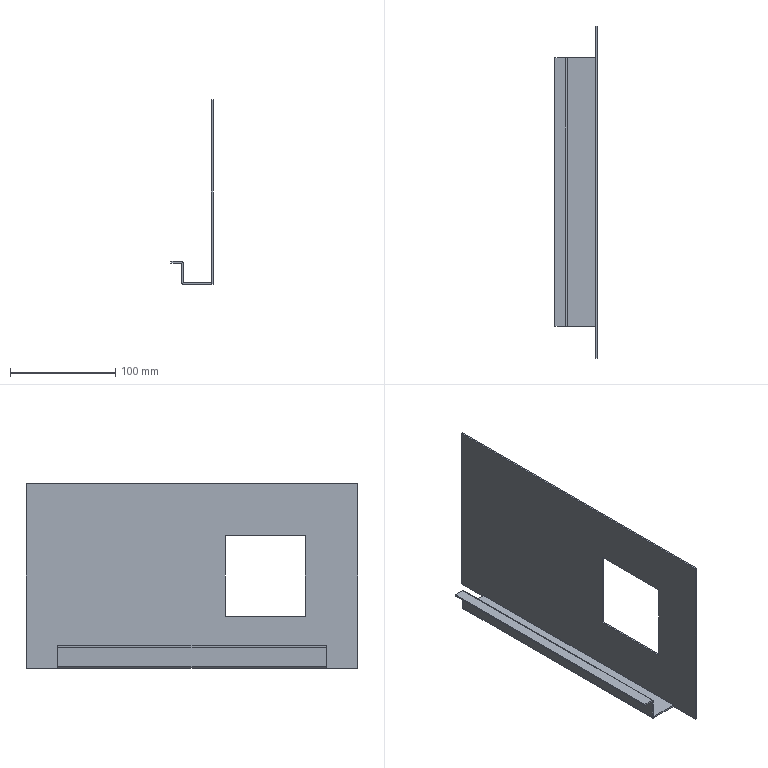Part | 1 solid | 42 faces | box 40 x 315 x 175 mm | volume 95980 mm3 | plane 36 | cylinder 6 | commonest cylinder face diameters 0.2 x3 3.2 x3
STEP:
#1=CARTESIAN_POINT('',(217.5,-127.5,-155.));
#2=VERTEX_POINT('',#1);
#3=CARTESIAN_POINT('',(217.5,-127.5,-153.5));
#4=VERTEX_POINT('',#3);
#5=CARTESIAN_POINT('',(217.5,-127.5,-663.884));
#6=DIRECTION('',(0.,0.,1.));
#7=VECTOR('',#6,1000.);
#8=LINE('',#5,#7);
#9=EDGE_CURVE('',#2,#4,#8,.T.);
#10=ORIENTED_EDGE('',*,*,#9,.T.);
#11=CARTESIAN_POINT('',(217.5,127.5,-153.5));
#12=VERTEX_POINT('',#11);
#13=CARTESIAN_POINT('',(217.5,-127.5,-153.5));
#14=DIRECTION('',(0.,1.,0.));
#15=VECTOR('',#14,1000.);
#16=LINE('',#13,#15);
#17=EDGE_CURVE('',#4,#12,#16,.T.);
#18=ORIENTED_EDGE('',*,*,#17,.T.);
#19=CARTESIAN_POINT('',(217.5,127.5,-155.));
#20=VERTEX_POINT('',#19);
#21=CARTESIAN_POINT('',(217.5,127.5,-663.884));
#22=DIRECTION('',(0.,0.,1.));
#23=VECTOR('',#22,1000.);
#24=LINE('',#21,#23);
#25=EDGE_CURVE('',#20,#12,#24,.T.);
#26=ORIENTED_EDGE('',*,*,#25,.F.);
#27=CARTESIAN_POINT('',(217.5,-127.5,-155.));
#28=DIRECTION('',(0.,1.,0.));
#29=VECTOR('',#28,1000.);
#30=LINE('',#27,#29);
#31=EDGE_CURVE('',#2,#20,#30,.T.);
#32=ORIENTED_EDGE('',*,*,#31,.F.);
#33=EDGE_LOOP('',(#10,#18,#26,#32));
#34=FACE_OUTER_BOUND('',#33,.T.);
#35=CARTESIAN_POINT('',(217.5,-127.5,-663.884));
#36=DIRECTION('',(1.,0.,0.));
#37=DIRECTION('',(0.,-1.,0.));
#38=AXIS2_PLACEMENT_3D('',#35,#36,#37);
#39=PLANE('',#38);
#40=ADVANCED_FACE('',(#34),#39,.F.);
#41=CARTESIAN_POINT('',(227.4,-127.5,-153.5));
#42=VERTEX_POINT('',#41);
#43=CARTESIAN_POINT('',(-2832.5,-127.5,-153.5));
#44=DIRECTION('',(1.,0.,0.));
#45=VECTOR('',#44,1000.);
#46=LINE('',#43,#45);
#47=EDGE_CURVE('',#4,#42,#46,.T.);
#48=ORIENTED_EDGE('',*,*,#47,.F.);
#49=ORIENTED_EDGE('',*,*,#9,.F.);
#50=CARTESIAN_POINT('',(227.4,-127.5,-155.));
#51=VERTEX_POINT('',#50);
#52=CARTESIAN_POINT('',(-2832.5,-127.5,-155.));
#53=DIRECTION('',(1.,0.,0.));
#54=VECTOR('',#53,1000.);
#55=LINE('',#52,#54);
#56=EDGE_CURVE('',#2,#51,#55,.T.);
#57=ORIENTED_EDGE('',*,*,#56,.T.);
#58=CARTESIAN_POINT('',(227.4,-127.5,-663.884));
#59=DIRECTION('',(0.,0.,1.));
#60=VECTOR('',#59,1000.);
#61=LINE('',#58,#60);
#62=EDGE_CURVE('',#51,#42,#61,.T.);
#63=ORIENTED_EDGE('',*,*,#62,.T.);
#64=EDGE_LOOP('',(#48,#49,#57,#63));
#65=FACE_OUTER_BOUND('',#64,.T.);
#66=CARTESIAN_POINT('',(-2832.5,-127.5,-663.884));
#67=DIRECTION('',(0.,-1.,0.));
#68=DIRECTION('',(-1.,0.,0.));
#69=AXIS2_PLACEMENT_3D('',#66,#67,#68);
#70=PLANE('',#69);
#71=ADVANCED_FACE('',(#65),#70,.T.);
#72=ORIENTED_EDGE('',*,*,#47,.T.);
#73=CARTESIAN_POINT('',(227.4,127.5,-153.5));
#74=VERTEX_POINT('',#73);
#75=CARTESIAN_POINT('',(227.4,-127.5,-153.5));
#76=DIRECTION('',(0.,1.,0.));
#77=VECTOR('',#76,1000.);
#78=LINE('',#75,#77);
#79=EDGE_CURVE('',#42,#74,#78,.T.);
#80=ORIENTED_EDGE('',*,*,#79,.T.);
#81=CARTESIAN_POINT('',(2832.5,127.5,-153.5));
#82=DIRECTION('',(-1.,0.,0.));
#83=VECTOR('',#82,1000.);
#84=LINE('',#81,#83);
#85=EDGE_CURVE('',#74,#12,#84,.T.);
#86=ORIENTED_EDGE('',*,*,#85,.T.);
#87=ORIENTED_EDGE('',*,*,#17,.F.);
#88=EDGE_LOOP('',(#72,#80,#86,#87));
#89=FACE_OUTER_BOUND('',#88,.T.);
#90=CARTESIAN_POINT('',(-2832.5,-127.5,-153.5));
#91=DIRECTION('',(0.,0.,-1.));
#92=DIRECTION('',(0.,-1.,0.));
#93=AXIS2_PLACEMENT_3D('',#90,#91,#92);
#94=PLANE('',#93);
#95=ADVANCED_FACE('',(#89),#94,.F.);
#96=ORIENTED_EDGE('',*,*,#85,.F.);
#97=CARTESIAN_POINT('',(227.4,127.5,-155.));
#98=VERTEX_POINT('',#97);
#99=CARTESIAN_POINT('',(227.4,127.5,-663.884));
#100=DIRECTION('',(0.,0.,1.));
#101=VECTOR('',#100,1000.);
#102=LINE('',#99,#101);
#103=EDGE_CURVE('',#98,#74,#102,.T.);
#104=ORIENTED_EDGE('',*,*,#103,.F.);
#105=CARTESIAN_POINT('',(2832.5,127.5,-155.));
#106=DIRECTION('',(-1.,0.,0.));
#107=VECTOR('',#106,1000.);
#108=LINE('',#105,#107);
#109=EDGE_CURVE('',#98,#20,#108,.T.);
#110=ORIENTED_EDGE('',*,*,#109,.T.);
#111=ORIENTED_EDGE('',*,*,#25,.T.);
#112=EDGE_LOOP('',(#96,#104,#110,#111));
#113=FACE_OUTER_BOUND('',#112,.T.);
#114=CARTESIAN_POINT('',(2832.5,127.5,-663.884));
#115=DIRECTION('',(0.,1.,0.));
#116=DIRECTION('',(1.,0.,0.));
#117=AXIS2_PLACEMENT_3D('',#114,#115,#116);
#118=PLANE('',#117);
#119=ADVANCED_FACE('',(#113),#118,.T.);
#120=CARTESIAN_POINT('',(227.4,-127.5,-155.));
#121=DIRECTION('',(0.,1.,0.));
#122=VECTOR('',#121,1000.);
#123=LINE('',#120,#122);
#124=EDGE_CURVE('',#51,#98,#123,.T.);
#125=ORIENTED_EDGE('',*,*,#124,.F.);
#126=ORIENTED_EDGE('',*,*,#56,.F.);
#127=ORIENTED_EDGE('',*,*,#31,.T.);
#128=ORIENTED_EDGE('',*,*,#109,.F.);
#129=EDGE_LOOP('',(#125,#126,#127,#128));
#130=FACE_OUTER_BOUND('',#129,.T.);
#131=CARTESIAN_POINT('',(-2832.5,-127.5,-155.));
#132=DIRECTION('',(0.,0.,-1.));
#133=DIRECTION('',(0.,-1.,0.));
#134=AXIS2_PLACEMENT_3D('',#131,#132,#133);
#135=PLANE('',#134);
#136=ADVANCED_FACE('',(#130),#135,.T.);
#137=CARTESIAN_POINT('',(227.5,-127.5,-173.4));
#138=VERTEX_POINT('',#137);
#139=CARTESIAN_POINT('',(227.5,-127.5,-155.1));
#140=VERTEX_POINT('',#139);
#141=CARTESIAN_POINT('',(227.5,-127.5,-175.));
#142=DIRECTION('',(0.,0.,1.));
#143=VECTOR('',#142,1000.);
#144=LINE('',#141,#143);
#145=EDGE_CURVE('',#138,#140,#144,.T.);
#146=ORIENTED_EDGE('',*,*,#145,.F.);
#147=CARTESIAN_POINT('',(229.,-127.5,-173.4));
#148=VERTEX_POINT('',#147);
#149=CARTESIAN_POINT('',(740.312,-127.5,-173.4));
#150=DIRECTION('',(-1.,0.,0.));
#151=VECTOR('',#150,1000.);
#152=LINE('',#149,#151);
#153=EDGE_CURVE('',#148,#138,#152,.T.);
#154=ORIENTED_EDGE('',*,*,#153,.F.);
#155=CARTESIAN_POINT('',(229.,-127.5,-155.1));
#156=VERTEX_POINT('',#155);
#157=CARTESIAN_POINT('',(229.,-127.5,-175.));
#158=DIRECTION('',(0.,0.,-1.));
#159=VECTOR('',#158,1000.);
#160=LINE('',#157,#159);
#161=EDGE_CURVE('',#156,#148,#160,.T.);
#162=ORIENTED_EDGE('',*,*,#161,.F.);
#163=CARTESIAN_POINT('',(740.312,-127.5,-155.1));
#164=DIRECTION('',(-1.,0.,0.));
#165=VECTOR('',#164,1000.);
#166=LINE('',#163,#165);
#167=EDGE_CURVE('',#156,#140,#166,.T.);
#168=ORIENTED_EDGE('',*,*,#167,.T.);
#169=EDGE_LOOP('',(#146,#154,#162,#168));
#170=FACE_OUTER_BOUND('',#169,.T.);
#171=CARTESIAN_POINT('',(740.312,-127.5,-175.));
#172=DIRECTION('',(0.,1.,0.));
#173=DIRECTION('',(0.,0.,-1.));
#174=AXIS2_PLACEMENT_3D('',#171,#172,#173);
#175=PLANE('',#174);
#176=ADVANCED_FACE('',(#170),#175,.F.);
#177=CARTESIAN_POINT('',(227.5,127.5,-155.1));
#178=VERTEX_POINT('',#177);
#179=CARTESIAN_POINT('',(227.5,127.5,-173.4));
#180=VERTEX_POINT('',#179);
#181=CARTESIAN_POINT('',(227.5,127.5,-175.));
#182=DIRECTION('',(0.,0.,-1.));
#183=VECTOR('',#182,1000.);
#184=LINE('',#181,#183);
#185=EDGE_CURVE('',#178,#180,#184,.T.);
#186=ORIENTED_EDGE('',*,*,#185,.F.);
#187=CARTESIAN_POINT('',(229.,127.5,-155.1));
#188=VERTEX_POINT('',#187);
#189=CARTESIAN_POINT('',(740.312,127.5,-155.1));
#190=DIRECTION('',(-1.,0.,0.));
#191=VECTOR('',#190,1000.);
#192=LINE('',#189,#191);
#193=EDGE_CURVE('',#188,#178,#192,.T.);
#194=ORIENTED_EDGE('',*,*,#193,.F.);
#195=CARTESIAN_POINT('',(229.,127.5,-173.4));
#196=VERTEX_POINT('',#195);
#197=CARTESIAN_POINT('',(229.,127.5,-175.));
#198=DIRECTION('',(0.,0.,-1.));
#199=VECTOR('',#198,1000.);
#200=LINE('',#197,#199);
#201=EDGE_CURVE('',#188,#196,#200,.T.);
#202=ORIENTED_EDGE('',*,*,#201,.T.);
#203=CARTESIAN_POINT('',(740.312,127.5,-173.4));
#204=DIRECTION('',(-1.,0.,0.));
#205=VECTOR('',#204,1000.);
#206=LINE('',#203,#205);
#207=EDGE_CURVE('',#196,#180,#206,.T.);
#208=ORIENTED_EDGE('',*,*,#207,.T.);
#209=EDGE_LOOP('',(#186,#194,#202,#208));
#210=FACE_OUTER_BOUND('',#209,.T.);
#211=CARTESIAN_POINT('',(740.312,127.5,-175.));
#212=DIRECTION('',(0.,-1.,0.));
#213=DIRECTION('',(0.,0.,1.));
#214=AXIS2_PLACEMENT_3D('',#211,#212,#213);
#215=PLANE('',#214);
#216=ADVANCED_FACE('',(#210),#215,.F.);
#217=ORIENTED_EDGE('',*,*,#201,.F.);
#218=CARTESIAN_POINT('',(229.,-127.5,-155.1));
#219=DIRECTION('',(0.,-1.,0.));
#220=VECTOR('',#219,1000.);
#221=LINE('',#218,#220);
#222=EDGE_CURVE('',#188,#156,#221,.T.);
#223=ORIENTED_EDGE('',*,*,#222,.T.);
#224=ORIENTED_EDGE('',*,*,#161,.T.);
#225=CARTESIAN_POINT('',(229.,127.5,-173.4));
#226=DIRECTION('',(0.,1.,0.));
#227=VECTOR('',#226,1000.);
#228=LINE('',#225,#227);
#229=EDGE_CURVE('',#148,#196,#228,.T.);
#230=ORIENTED_EDGE('',*,*,#229,.T.);
#231=EDGE_LOOP('',(#217,#223,#224,#230));
#232=FACE_OUTER_BOUND('',#231,.T.);
#233=CARTESIAN_POINT('',(229.,-2732.5,-175.));
#234=DIRECTION('',(-1.,0.,0.));
#235=DIRECTION('',(0.,0.,-1.));
#236=AXIS2_PLACEMENT_3D('',#233,#234,#235);
#237=PLANE('',#236);
#238=ADVANCED_FACE('',(#232),#237,.F.);
#239=CARTESIAN_POINT('',(227.5,-127.5,-155.1));
#240=DIRECTION('',(0.,-1.,0.));
#241=VECTOR('',#240,1000.);
#242=LINE('',#239,#241);
#243=EDGE_CURVE('',#178,#140,#242,.T.);
#244=ORIENTED_EDGE('',*,*,#243,.F.);
#245=ORIENTED_EDGE('',*,*,#185,.T.);
#246=CARTESIAN_POINT('',(227.5,127.5,-173.4));
#247=DIRECTION('',(0.,1.,0.));
#248=VECTOR('',#247,1000.);
#249=LINE('',#246,#248);
#250=EDGE_CURVE('',#138,#180,#249,.T.);
#251=ORIENTED_EDGE('',*,*,#250,.F.);
#252=ORIENTED_EDGE('',*,*,#145,.T.);
#253=EDGE_LOOP('',(#244,#245,#251,#252));
#254=FACE_OUTER_BOUND('',#253,.T.);
#255=CARTESIAN_POINT('',(227.5,-127.5,-175.));
#256=DIRECTION('',(-1.,0.,0.));
#257=DIRECTION('',(0.,0.,1.));
#258=AXIS2_PLACEMENT_3D('',#255,#256,#257);
#259=PLANE('',#258);
#260=ADVANCED_FACE('',(#254),#259,.T.);
#261=CARTESIAN_POINT('',(256.,127.65,-173.25));
#262=VERTEX_POINT('',#261);
#263=CARTESIAN_POINT('',(257.5,127.65,-173.25));
#264=VERTEX_POINT('',#263);
#265=CARTESIAN_POINT('',(-464.694,127.65,-173.25));
#266=DIRECTION('',(1.,0.,0.));
#267=VECTOR('',#266,1000.);
#268=LINE('',#265,#267);
#269=EDGE_CURVE('',#262,#264,#268,.T.);
#270=ORIENTED_EDGE('',*,*,#269,.T.);
#271=CARTESIAN_POINT('',(257.5,127.5,-173.25));
#272=VERTEX_POINT('',#271);
#273=CARTESIAN_POINT('',(257.5,-2732.5,-173.25));
#274=DIRECTION('',(0.,-1.,0.));
#275=VECTOR('',#274,1000.);
#276=LINE('',#273,#275);
#277=EDGE_CURVE('',#264,#272,#276,.T.);
#278=ORIENTED_EDGE('',*,*,#277,.T.);
#279=CARTESIAN_POINT('',(256.,127.5,-173.25));
#280=VERTEX_POINT('',#279);
#281=CARTESIAN_POINT('',(-464.694,127.5,-173.25));
#282=DIRECTION('',(1.,0.,0.));
#283=VECTOR('',#282,1000.);
#284=LINE('',#281,#283);
#285=EDGE_CURVE('',#280,#272,#284,.T.);
#286=ORIENTED_EDGE('',*,*,#285,.F.);
#287=CARTESIAN_POINT('',(256.,-156.3,-173.25));
#288=DIRECTION('',(0.,-1.,0.));
#289=VECTOR('',#288,1000.);
#290=LINE('',#287,#289);
#291=EDGE_CURVE('',#262,#280,#290,.T.);
#292=ORIENTED_EDGE('',*,*,#291,.F.);
#293=EDGE_LOOP('',(#270,#278,#286,#292));
#294=FACE_OUTER_BOUND('',#293,.T.);
#295=CARTESIAN_POINT('',(-464.694,-156.3,-173.25));
#296=DIRECTION('',(0.,0.,1.));
#297=DIRECTION('',(0.,-1.,0.));
#298=AXIS2_PLACEMENT_3D('',#295,#296,#297);
#299=PLANE('',#298);
#300=ADVANCED_FACE('',(#294),#299,.F.);
#301=CARTESIAN_POINT('',(256.,127.65,-175.));
#302=VERTEX_POINT('',#301);
#303=CARTESIAN_POINT('',(257.5,127.65,-175.));
#304=VERTEX_POINT('',#303);
#305=CARTESIAN_POINT('',(-464.694,127.65,-175.));
#306=DIRECTION('',(1.,0.,0.));
#307=VECTOR('',#306,1000.);
#308=LINE('',#305,#307);
#309=EDGE_CURVE('',#302,#304,#308,.T.);
#310=ORIENTED_EDGE('',*,*,#309,.T.);
#311=CARTESIAN_POINT('',(257.5,127.65,-173.063));
#312=DIRECTION('',(0.,0.,1.));
#313=VECTOR('',#312,1000.);
#314=LINE('',#311,#313);
#315=EDGE_CURVE('',#304,#264,#314,.T.);
#316=ORIENTED_EDGE('',*,*,#315,.T.);
#317=ORIENTED_EDGE('',*,*,#269,.F.);
#318=CARTESIAN_POINT('',(256.,127.65,-173.8));
#319=DIRECTION('',(0.,0.,1.));
#320=VECTOR('',#319,1000.);
#321=LINE('',#318,#320);
#322=EDGE_CURVE('',#302,#262,#321,.T.);
#323=ORIENTED_EDGE('',*,*,#322,.F.);
#324=EDGE_LOOP('',(#310,#316,#317,#323));
#325=FACE_OUTER_BOUND('',#324,.T.);
#326=CARTESIAN_POINT('',(-464.694,127.65,-173.8));
#327=DIRECTION('',(0.,1.,0.));
#328=DIRECTION('',(0.,0.,1.));
#329=AXIS2_PLACEMENT_3D('',#326,#327,#328);
#330=PLANE('',#329);
#331=ADVANCED_FACE('',(#325),#330,.F.);
#332=CARTESIAN_POINT('',(257.5,157.5,-175.));
#333=VERTEX_POINT('',#332);
#334=CARTESIAN_POINT('',(257.5,-2732.5,-175.));
#335=DIRECTION('',(0.,1.,0.));
#336=VECTOR('',#335,1000.);
#337=LINE('',#334,#336);
#338=EDGE_CURVE('',#304,#333,#337,.T.);
#339=ORIENTED_EDGE('',*,*,#338,.F.);
#340=ORIENTED_EDGE('',*,*,#309,.F.);
#341=CARTESIAN_POINT('',(256.,157.5,-175.));
#342=VERTEX_POINT('',#341);
#343=CARTESIAN_POINT('',(256.,2732.5,-175.));
#344=DIRECTION('',(0.,1.,0.));
#345=VECTOR('',#344,1000.);
#346=LINE('',#343,#345);
#347=EDGE_CURVE('',#302,#342,#346,.T.);
#348=ORIENTED_EDGE('',*,*,#347,.T.);
#349=CARTESIAN_POINT('',(-464.694,157.5,-175.));
#350=DIRECTION('',(1.,0.,0.));
#351=VECTOR('',#350,1000.);
#352=LINE('',#349,#351);
#353=EDGE_CURVE('',#342,#333,#352,.T.);
#354=ORIENTED_EDGE('',*,*,#353,.T.);
#355=EDGE_LOOP('',(#339,#340,#348,#354));
#356=FACE_OUTER_BOUND('',#355,.T.);
#357=CARTESIAN_POINT('',(-464.694,2732.5,-175.));
#358=DIRECTION('',(0.,0.,-1.));
#359=DIRECTION('',(-1.,0.,0.));
#360=AXIS2_PLACEMENT_3D('',#357,#358,#359);
#361=PLANE('',#360);
#362=ADVANCED_FACE('',(#356),#361,.T.);
#363=CARTESIAN_POINT('',(256.,157.5,0.));
#364=VERTEX_POINT('',#363);
#365=CARTESIAN_POINT('',(257.5,157.5,0.));
#366=VERTEX_POINT('',#365);
#367=CARTESIAN_POINT('',(-464.694,157.5,0.));
#368=DIRECTION('',(1.,0.,0.));
#369=VECTOR('',#368,1000.);
#370=LINE('',#367,#369);
#371=EDGE_CURVE('',#364,#366,#370,.T.);
#372=ORIENTED_EDGE('',*,*,#371,.T.);
#373=CARTESIAN_POINT('',(257.5,157.5,-173.063));
#374=DIRECTION('',(0.,0.,-1.));
#375=VECTOR('',#374,1000.);
#376=LINE('',#373,#375);
#377=EDGE_CURVE('',#366,#333,#376,.T.);
#378=ORIENTED_EDGE('',*,*,#377,.T.);
#379=ORIENTED_EDGE('',*,*,#353,.F.);
#380=CARTESIAN_POINT('',(256.,157.5,-173.063));
#381=DIRECTION('',(0.,0.,-1.));
#382=VECTOR('',#381,1000.);
#383=LINE('',#380,#382);
#384=EDGE_CURVE('',#364,#342,#383,.T.);
#385=ORIENTED_EDGE('',*,*,#384,.F.);
#386=EDGE_LOOP('',(#372,#378,#379,#385));
#387=FACE_OUTER_BOUND('',#386,.T.);
#388=CARTESIAN_POINT('',(-464.694,157.5,-173.063));
#389=DIRECTION('',(0.,-1.,0.));
#390=DIRECTION('',(1.,0.,0.));
#391=AXIS2_PLACEMENT_3D('',#388,#389,#390);
#392=PLANE('',#391);
#393=ADVANCED_FACE('',(#387),#392,.F.);
#394=CARTESIAN_POINT('',(257.5,-157.5,0.));
#395=VERTEX_POINT('',#394);
#396=CARTESIAN_POINT('',(257.5,-2732.5,0.));
#397=DIRECTION('',(0.,1.,0.));
#398=VECTOR('',#397,1000.);
#399=LINE('',#396,#398);
#400=EDGE_CURVE('',#395,#366,#399,.T.);
#401=ORIENTED_EDGE('',*,*,#400,.T.);
#402=ORIENTED_EDGE('',*,*,#371,.F.);
#403=CARTESIAN_POINT('',(256.,-157.5,0.));
#404=VERTEX_POINT('',#403);
#405=CARTESIAN_POINT('',(256.,0.,0.));
#406=DIRECTION('',(0.,-1.,0.));
#407=VECTOR('',#406,1000.);
#408=LINE('',#405,#407);
#409=EDGE_CURVE('',#364,#404,#408,.T.);
#410=ORIENTED_EDGE('',*,*,#409,.T.);
#411=CARTESIAN_POINT('',(-464.694,-157.5,0.));
#412=DIRECTION('',(1.,0.,0.));
#413=VECTOR('',#412,1000.);
#414=LINE('',#411,#413);
#415=EDGE_CURVE('',#404,#395,#414,.T.);
#416=ORIENTED_EDGE('',*,*,#415,.T.);
#417=EDGE_LOOP('',(#401,#402,#410,#416));
#418=FACE_OUTER_BOUND('',#417,.T.);
#419=CARTESIAN_POINT('',(-464.694,0.,0.));
#420=DIRECTION('',(0.,0.,1.));
#421=DIRECTION('',(1.,0.,0.));
#422=AXIS2_PLACEMENT_3D('',#419,#420,#421);
#423=PLANE('',#422);
#424=ADVANCED_FACE('',(#418),#423,.T.);
#425=CARTESIAN_POINT('',(256.,-157.5,-175.));
#426=VERTEX_POINT('',#425);
#427=CARTESIAN_POINT('',(257.5,-157.5,-175.));
#428=VERTEX_POINT('',#427);
#429=CARTESIAN_POINT('',(-464.694,-157.5,-175.));
#430=DIRECTION('',(1.,0.,0.));
#431=VECTOR('',#430,1000.);
#432=LINE('',#429,#431);
#433=EDGE_CURVE('',#426,#428,#432,.T.);
#434=ORIENTED_EDGE('',*,*,#433,.T.);
#435=CARTESIAN_POINT('',(257.5,-157.5,-173.063));
#436=DIRECTION('',(0.,0.,-1.));
#437=VECTOR('',#436,1000.);
#438=LINE('',#435,#437);
#439=EDGE_CURVE('',#395,#428,#438,.T.);
#440=ORIENTED_EDGE('',*,*,#439,.F.);
#441=ORIENTED_EDGE('',*,*,#415,.F.);
#442=CARTESIAN_POINT('',(256.,-157.5,-173.063));
#443=DIRECTION('',(0.,0.,1.));
#444=VECTOR('',#443,1000.);
#445=LINE('',#442,#444);
#446=EDGE_CURVE('',#426,#404,#445,.T.);
#447=ORIENTED_EDGE('',*,*,#446,.F.);
#448=EDGE_LOOP('',(#434,#440,#441,#447));
#449=FACE_OUTER_BOUND('',#448,.T.);
#450=CARTESIAN_POINT('',(-464.694,-157.5,-173.063));
#451=DIRECTION('',(0.,1.,0.));
#452=DIRECTION('',(-1.,0.,0.));
#453=AXIS2_PLACEMENT_3D('',#450,#451,#452);
#454=PLANE('',#453);
#455=ADVANCED_FACE('',(#449),#454,.F.);
#456=CARTESIAN_POINT('',(257.5,-127.65,-175.));
#457=VERTEX_POINT('',#456);
#458=CARTESIAN_POINT('',(257.5,-2732.5,-175.));
#459=DIRECTION('',(0.,1.,0.));
#460=VECTOR('',#459,1000.);
#461=LINE('',#458,#460);
#462=EDGE_CURVE('',#428,#457,#461,.T.);
#463=ORIENTED_EDGE('',*,*,#462,.F.);
#464=ORIENTED_EDGE('',*,*,#433,.F.);
#465=CARTESIAN_POINT('',(256.,-127.65,-175.));
#466=VERTEX_POINT('',#465);
#467=CARTESIAN_POINT('',(256.,2732.5,-175.));
#468=DIRECTION('',(0.,1.,0.));
#469=VECTOR('',#468,1000.);
#470=LINE('',#467,#469);
#471=EDGE_CURVE('',#426,#466,#470,.T.);
#472=ORIENTED_EDGE('',*,*,#471,.T.);
#473=CARTESIAN_POINT('',(-464.694,-127.65,-175.));
#474=DIRECTION('',(1.,0.,0.));
#475=VECTOR('',#474,1000.);
#476=LINE('',#473,#475);
#477=EDGE_CURVE('',#466,#457,#476,.T.);
#478=ORIENTED_EDGE('',*,*,#477,.T.);
#479=EDGE_LOOP('',(#463,#464,#472,#478));
#480=FACE_OUTER_BOUND('',#479,.T.);
#481=CARTESIAN_POINT('',(-464.694,2732.5,-175.));
#482=DIRECTION('',(0.,0.,-1.));
#483=DIRECTION('',(-1.,0.,0.));
#484=AXIS2_PLACEMENT_3D('',#481,#482,#483);
#485=PLANE('',#484);
#486=ADVANCED_FACE('',(#480),#485,.T.);
#487=CARTESIAN_POINT('',(256.,-127.65,-173.25));
#488=VERTEX_POINT('',#487);
#489=CARTESIAN_POINT('',(257.5,-127.65,-173.25));
#490=VERTEX_POINT('',#489);
#491=CARTESIAN_POINT('',(-464.694,-127.65,-173.25));
#492=DIRECTION('',(1.,0.,0.));
#493=VECTOR('',#492,1000.);
#494=LINE('',#491,#493);
#495=EDGE_CURVE('',#488,#490,#494,.T.);
#496=ORIENTED_EDGE('',*,*,#495,.T.);
#497=CARTESIAN_POINT('',(257.5,-127.65,-173.063));
#498=DIRECTION('',(0.,0.,-1.));
#499=VECTOR('',#498,1000.);
#500=LINE('',#497,#499);
#501=EDGE_CURVE('',#490,#457,#500,.T.);
#502=ORIENTED_EDGE('',*,*,#501,.T.);
#503=ORIENTED_EDGE('',*,*,#477,.F.);
#504=CARTESIAN_POINT('',(256.,-127.65,-173.8));
#505=DIRECTION('',(0.,0.,-1.));
#506=VECTOR('',#505,1000.);
#507=LINE('',#504,#506);
#508=EDGE_CURVE('',#488,#466,#507,.T.);
#509=ORIENTED_EDGE('',*,*,#508,.F.);
#510=EDGE_LOOP('',(#496,#502,#503,#509));
#511=FACE_OUTER_BOUND('',#510,.T.);
#512=CARTESIAN_POINT('',(-464.694,-127.65,-173.8));
#513=DIRECTION('',(0.,-1.,0.));
#514=DIRECTION('',(0.,0.,-1.));
#515=AXIS2_PLACEMENT_3D('',#512,#513,#514);
#516=PLANE('',#515);
#517=ADVANCED_FACE('',(#511),#516,.F.);
#518=CARTESIAN_POINT('',(256.,-127.5,-173.25));
#519=VERTEX_POINT('',#518);
#520=CARTESIAN_POINT('',(257.5,-127.5,-173.25));
#521=VERTEX_POINT('',#520);
#522=CARTESIAN_POINT('',(-464.694,-127.5,-173.25));
#523=DIRECTION('',(1.,0.,0.));
#524=VECTOR('',#523,1000.);
#525=LINE('',#522,#524);
#526=EDGE_CURVE('',#519,#521,#525,.T.);
#527=ORIENTED_EDGE('',*,*,#526,.T.);
#528=CARTESIAN_POINT('',(257.5,-2732.5,-173.25));
#529=DIRECTION('',(0.,-1.,0.));
#530=VECTOR('',#529,1000.);
#531=LINE('',#528,#530);
#532=EDGE_CURVE('',#521,#490,#531,.T.);
#533=ORIENTED_EDGE('',*,*,#532,.T.);
#534=ORIENTED_EDGE('',*,*,#495,.F.);
#535=CARTESIAN_POINT('',(256.,-156.3,-173.25));
#536=DIRECTION('',(0.,-1.,0.));
#537=VECTOR('',#536,1000.);
#538=LINE('',#535,#537);
#539=EDGE_CURVE('',#519,#488,#538,.T.);
#540=ORIENTED_EDGE('',*,*,#539,.F.);
#541=EDGE_LOOP('',(#527,#533,#534,#540));
#542=FACE_OUTER_BOUND('',#541,.T.);
#543=CARTESIAN_POINT('',(-464.694,-156.3,-173.25));
#544=DIRECTION('',(0.,0.,1.));
#545=DIRECTION('',(0.,-1.,0.));
#546=AXIS2_PLACEMENT_3D('',#543,#544,#545);
#547=PLANE('',#546);
#548=ADVANCED_FACE('',(#542),#547,.F.);
#549=CARTESIAN_POINT('',(257.5,-107.5,-49.5));
#550=VERTEX_POINT('',#549);
#551=CARTESIAN_POINT('',(257.5,-107.5,-125.5));
#552=VERTEX_POINT('',#551);
#553=CARTESIAN_POINT('',(257.5,-107.5,-125.5));
#554=DIRECTION('',(0.,0.,-1.));
#555=VECTOR('',#554,1000.);
#556=LINE('',#553,#555);
#557=EDGE_CURVE('',#550,#552,#556,.T.);
#558=ORIENTED_EDGE('',*,*,#557,.T.);
#559=CARTESIAN_POINT('',(256.,-107.5,-125.5));
#560=VERTEX_POINT('',#559);
#561=CARTESIAN_POINT('',(256.3,-107.5,-125.5));
#562=DIRECTION('',(1.,0.,0.));
#563=VECTOR('',#562,1000.);
#564=LINE('',#561,#563);
#565=EDGE_CURVE('',#560,#552,#564,.T.);
#566=ORIENTED_EDGE('',*,*,#565,.F.);
#567=CARTESIAN_POINT('',(256.,-107.5,-49.5));
#568=VERTEX_POINT('',#567);
#569=CARTESIAN_POINT('',(256.,-107.5,-125.5));
#570=DIRECTION('',(0.,0.,-1.));
#571=VECTOR('',#570,1000.);
#572=LINE('',#569,#571);
#573=EDGE_CURVE('',#568,#560,#572,.T.);
#574=ORIENTED_EDGE('',*,*,#573,.F.);
#575=CARTESIAN_POINT('',(256.3,-107.5,-49.5));
#576=DIRECTION('',(1.,0.,0.));
#577=VECTOR('',#576,1000.);
#578=LINE('',#575,#577);
#579=EDGE_CURVE('',#568,#550,#578,.T.);
#580=ORIENTED_EDGE('',*,*,#579,.T.);
#581=EDGE_LOOP('',(#558,#566,#574,#580));
#582=FACE_OUTER_BOUND('',#581,.T.);
#583=CARTESIAN_POINT('',(256.3,-107.5,-125.5));
#584=DIRECTION('',(0.,-1.,0.));
#585=DIRECTION('',(0.,0.,-1.));
#586=AXIS2_PLACEMENT_3D('',#583,#584,#585);
#587=PLANE('',#586);
#588=ADVANCED_FACE('',(#582),#587,.F.);
#589=CARTESIAN_POINT('',(257.5,-31.5,-49.5));
#590=VERTEX_POINT('',#589);
#591=CARTESIAN_POINT('',(257.5,-107.5,-49.5));
#592=DIRECTION('',(0.,-1.,0.));
#593=VECTOR('',#592,1000.);
#594=LINE('',#591,#593);
#595=EDGE_CURVE('',#590,#550,#594,.T.);
#596=ORIENTED_EDGE('',*,*,#595,.T.);
#597=ORIENTED_EDGE('',*,*,#579,.F.);
#598=CARTESIAN_POINT('',(256.,-31.5,-49.5));
#599=VERTEX_POINT('',#598);
#600=CARTESIAN_POINT('',(256.,-107.5,-49.5));
#601=DIRECTION('',(0.,-1.,0.));
#602=VECTOR('',#601,1000.);
#603=LINE('',#600,#602);
#604=EDGE_CURVE('',#599,#568,#603,.T.);
#605=ORIENTED_EDGE('',*,*,#604,.F.);
#606=CARTESIAN_POINT('',(256.3,-31.5,-49.5));
#607=DIRECTION('',(1.,0.,0.));
#608=VECTOR('',#607,1000.);
#609=LINE('',#606,#608);
#610=EDGE_CURVE('',#599,#590,#609,.T.);
#611=ORIENTED_EDGE('',*,*,#610,.T.);
#612=EDGE_LOOP('',(#596,#597,#605,#611));
#613=FACE_OUTER_BOUND('',#612,.T.);
#614=CARTESIAN_POINT('',(256.3,-107.5,-49.5));
#615=DIRECTION('',(0.,0.,1.));
#616=DIRECTION('',(0.,-1.,0.));
#617=AXIS2_PLACEMENT_3D('',#614,#615,#616);
#618=PLANE('',#617);
#619=ADVANCED_FACE('',(#613),#618,.F.);
#620=CARTESIAN_POINT('',(257.5,-31.5,-125.5));
#621=VERTEX_POINT('',#620);
#622=CARTESIAN_POINT('',(257.5,-31.5,-125.5));
#623=DIRECTION('',(0.,0.,1.));
#624=VECTOR('',#623,1000.);
#625=LINE('',#622,#624);
#626=EDGE_CURVE('',#621,#590,#625,.T.);
#627=ORIENTED_EDGE('',*,*,#626,.T.);
#628=ORIENTED_EDGE('',*,*,#610,.F.);
#629=CARTESIAN_POINT('',(256.,-31.5,-125.5));
#630=VERTEX_POINT('',#629);
#631=CARTESIAN_POINT('',(256.,-31.5,-125.5));
#632=DIRECTION('',(0.,0.,1.));
#633=VECTOR('',#632,1000.);
#634=LINE('',#631,#633);
#635=EDGE_CURVE('',#630,#599,#634,.T.);
#636=ORIENTED_EDGE('',*,*,#635,.F.);
#637=CARTESIAN_POINT('',(256.3,-31.5,-125.5));
#638=DIRECTION('',(1.,0.,0.));
#639=VECTOR('',#638,1000.);
#640=LINE('',#637,#639);
#641=EDGE_CURVE('',#630,#621,#640,.T.);
#642=ORIENTED_EDGE('',*,*,#641,.T.);
#643=EDGE_LOOP('',(#627,#628,#636,#642));
#644=FACE_OUTER_BOUND('',#643,.T.);
#645=CARTESIAN_POINT('',(256.3,-31.5,-125.5));
#646=DIRECTION('',(0.,1.,0.));
#647=DIRECTION('',(0.,0.,1.));
#648=AXIS2_PLACEMENT_3D('',#645,#646,#647);
#649=PLANE('',#648);
#650=ADVANCED_FACE('',(#644),#649,.F.);
#651=CARTESIAN_POINT('',(257.5,-107.5,-125.5));
#652=DIRECTION('',(0.,1.,0.));
#653=VECTOR('',#652,1000.);
#654=LINE('',#651,#653);
#655=EDGE_CURVE('',#552,#621,#654,.T.);
#656=ORIENTED_EDGE('',*,*,#655,.T.);
#657=ORIENTED_EDGE('',*,*,#641,.F.);
#658=CARTESIAN_POINT('',(256.,-107.5,-125.5));
#659=DIRECTION('',(0.,1.,0.));
#660=VECTOR('',#659,1000.);
#661=LINE('',#658,#660);
#662=EDGE_CURVE('',#560,#630,#661,.T.);
#663=ORIENTED_EDGE('',*,*,#662,.F.);
#664=ORIENTED_EDGE('',*,*,#565,.T.);
#665=EDGE_LOOP('',(#656,#657,#663,#664));
#666=FACE_OUTER_BOUND('',#665,.T.);
#667=CARTESIAN_POINT('',(256.3,-107.5,-125.5));
#668=DIRECTION('',(0.,0.,-1.));
#669=DIRECTION('',(-1.,0.,0.));
#670=AXIS2_PLACEMENT_3D('',#667,#668,#669);
#671=PLANE('',#670);
#672=ADVANCED_FACE('',(#666),#671,.F.);
#673=ORIENTED_EDGE('',*,*,#285,.T.);
#674=CARTESIAN_POINT('',(257.5,127.5,-173.4));
#675=VERTEX_POINT('',#674);
#676=CARTESIAN_POINT('',(257.5,127.5,-173.063));
#677=DIRECTION('',(0.,0.,-1.));
#678=VECTOR('',#677,1000.);
#679=LINE('',#676,#678);
#680=EDGE_CURVE('',#272,#675,#679,.T.);
#681=ORIENTED_EDGE('',*,*,#680,.T.);
#682=CARTESIAN_POINT('',(256.,127.5,-173.4));
#683=VERTEX_POINT('',#682);
#684=CARTESIAN_POINT('',(-464.694,127.5,-173.4));
#685=DIRECTION('',(1.,0.,0.));
#686=VECTOR('',#685,1000.);
#687=LINE('',#684,#686);
#688=EDGE_CURVE('',#683,#675,#687,.T.);
#689=ORIENTED_EDGE('',*,*,#688,.F.);
#690=CARTESIAN_POINT('',(256.,127.5,-173.8));
#691=DIRECTION('',(0.,0.,-1.));
#692=VECTOR('',#691,1000.);
#693=LINE('',#690,#692);
#694=EDGE_CURVE('',#280,#683,#693,.T.);
#695=ORIENTED_EDGE('',*,*,#694,.F.);
#696=EDGE_LOOP('',(#673,#681,#689,#695));
#697=FACE_OUTER_BOUND('',#696,.T.);
#698=CARTESIAN_POINT('',(-464.694,127.5,-173.8));
#699=DIRECTION('',(0.,-1.,0.));
#700=DIRECTION('',(0.,0.,-1.));
#701=AXIS2_PLACEMENT_3D('',#698,#699,#700);
#702=PLANE('',#701);
#703=ADVANCED_FACE('',(#697),#702,.F.);
#704=ORIENTED_EDGE('',*,*,#626,.F.);
#705=ORIENTED_EDGE('',*,*,#655,.F.);
#706=ORIENTED_EDGE('',*,*,#557,.F.);
#707=ORIENTED_EDGE('',*,*,#595,.F.);
#708=EDGE_LOOP('',(#704,#705,#706,#707));
#709=FACE_BOUND('',#708,.T.);
#710=CARTESIAN_POINT('',(257.5,-127.5,-173.4));
#711=VERTEX_POINT('',#710);
#712=CARTESIAN_POINT('',(257.5,127.5,-173.4));
#713=DIRECTION('',(0.,-1.,0.));
#714=VECTOR('',#713,1000.);
#715=LINE('',#712,#714);
#716=EDGE_CURVE('',#675,#711,#715,.T.);
#717=ORIENTED_EDGE('',*,*,#716,.F.);
#718=ORIENTED_EDGE('',*,*,#680,.F.);
#719=ORIENTED_EDGE('',*,*,#277,.F.);
#720=ORIENTED_EDGE('',*,*,#315,.F.);
#721=ORIENTED_EDGE('',*,*,#338,.T.);
#722=ORIENTED_EDGE('',*,*,#377,.F.);
#723=ORIENTED_EDGE('',*,*,#400,.F.);
#724=ORIENTED_EDGE('',*,*,#439,.T.);
#725=ORIENTED_EDGE('',*,*,#462,.T.);
#726=ORIENTED_EDGE('',*,*,#501,.F.);
#727=ORIENTED_EDGE('',*,*,#532,.F.);
#728=CARTESIAN_POINT('',(257.5,-127.5,-173.063));
#729=DIRECTION('',(0.,0.,1.));
#730=VECTOR('',#729,1000.);
#731=LINE('',#728,#730);
#732=EDGE_CURVE('',#711,#521,#731,.T.);
#733=ORIENTED_EDGE('',*,*,#732,.F.);
#734=EDGE_LOOP('',(#717,#718,#719,#720,#721,#722,#723,#724,#725,#726,#727,#733));
#735=FACE_OUTER_BOUND('',#734,.T.);
#736=CARTESIAN_POINT('',(257.5,-2732.5,-173.063));
#737=DIRECTION('',(-1.,0.,0.));
#738=DIRECTION('',(0.,-1.,0.));
#739=AXIS2_PLACEMENT_3D('',#736,#737,#738);
#740=PLANE('',#739);
#741=ADVANCED_FACE('',(#709,#735),#740,.F.);
#742=CARTESIAN_POINT('',(256.,-127.5,-173.4));
#743=VERTEX_POINT('',#742);
#744=CARTESIAN_POINT('',(-464.694,-127.5,-173.4));
#745=DIRECTION('',(1.,0.,0.));
#746=VECTOR('',#745,1000.);
#747=LINE('',#744,#746);
#748=EDGE_CURVE('',#743,#711,#747,.T.);
#749=ORIENTED_EDGE('',*,*,#748,.T.);
#750=ORIENTED_EDGE('',*,*,#732,.T.);
#751=ORIENTED_EDGE('',*,*,#526,.F.);
#752=CARTESIAN_POINT('',(256.,-127.5,-173.8));
#753=DIRECTION('',(0.,0.,1.));
#754=VECTOR('',#753,1000.);
#755=LINE('',#752,#754);
#756=EDGE_CURVE('',#743,#519,#755,.T.);
#757=ORIENTED_EDGE('',*,*,#756,.F.);
#758=EDGE_LOOP('',(#749,#750,#751,#757));
#759=FACE_OUTER_BOUND('',#758,.T.);
#760=CARTESIAN_POINT('',(-464.694,-127.5,-173.8));
#761=DIRECTION('',(0.,1.,0.));
#762=DIRECTION('',(0.,0.,1.));
#763=AXIS2_PLACEMENT_3D('',#760,#761,#762);
#764=PLANE('',#763);
#765=ADVANCED_FACE('',(#759),#764,.F.);
#766=ORIENTED_EDGE('',*,*,#662,.T.);
#767=ORIENTED_EDGE('',*,*,#635,.T.);
#768=ORIENTED_EDGE('',*,*,#604,.T.);
#769=ORIENTED_EDGE('',*,*,#573,.T.);
#770=EDGE_LOOP('',(#766,#767,#768,#769));
#771=FACE_BOUND('',#770,.T.);
#772=ORIENTED_EDGE('',*,*,#694,.T.);
#773=CARTESIAN_POINT('',(256.,127.5,-173.4));
#774=DIRECTION('',(0.,-1.,0.));
#775=VECTOR('',#774,1000.);
#776=LINE('',#773,#775);
#777=EDGE_CURVE('',#683,#743,#776,.T.);
#778=ORIENTED_EDGE('',*,*,#777,.T.);
#779=ORIENTED_EDGE('',*,*,#756,.T.);
#780=ORIENTED_EDGE('',*,*,#539,.T.);
#781=ORIENTED_EDGE('',*,*,#508,.T.);
#782=ORIENTED_EDGE('',*,*,#471,.F.);
#783=ORIENTED_EDGE('',*,*,#446,.T.);
#784=ORIENTED_EDGE('',*,*,#409,.F.);
#785=ORIENTED_EDGE('',*,*,#384,.T.);
#786=ORIENTED_EDGE('',*,*,#347,.F.);
#787=ORIENTED_EDGE('',*,*,#322,.T.);
#788=ORIENTED_EDGE('',*,*,#291,.T.);
#789=EDGE_LOOP('',(#772,#778,#779,#780,#781,#782,#783,#784,#785,#786,#787,#788));
#790=FACE_OUTER_BOUND('',#789,.T.);
#791=CARTESIAN_POINT('',(256.,-156.3,-173.8));
#792=DIRECTION('',(-1.,0.,0.));
#793=DIRECTION('',(0.,-1.,0.));
#794=AXIS2_PLACEMENT_3D('',#791,#792,#793);
#795=PLANE('',#794);
#796=ADVANCED_FACE('',(#771,#790),#795,.T.);
#797=CARTESIAN_POINT('',(255.9,127.5,-173.5));
#798=VERTEX_POINT('',#797);
#799=CARTESIAN_POINT('',(255.9,127.5,-175.));
#800=VERTEX_POINT('',#799);
#801=CARTESIAN_POINT('',(255.9,127.5,339.309));
#802=DIRECTION('',(0.,0.,-1.));
#803=VECTOR('',#802,1000.);
#804=LINE('',#801,#803);
#805=EDGE_CURVE('',#798,#800,#804,.T.);
#806=ORIENTED_EDGE('',*,*,#805,.F.);
#807=CARTESIAN_POINT('',(255.9,127.5,-173.4));
#808=DIRECTION('',(0.,-1.,0.));
#809=DIRECTION('',(0.,0.,-1.));
#810=AXIS2_PLACEMENT_3D('',#807,#808,#809);
#811=CIRCLE('',#810,0.1);
#812=EDGE_CURVE('',#798,#683,#811,.T.);
#813=ORIENTED_EDGE('',*,*,#812,.T.);
#814=ORIENTED_EDGE('',*,*,#688,.T.);
#815=CARTESIAN_POINT('',(255.9,127.5,-173.4));
#816=DIRECTION('',(0.,-1.,0.));
#817=DIRECTION('',(0.,0.,-1.));
#818=AXIS2_PLACEMENT_3D('',#815,#816,#817);
#819=CIRCLE('',#818,1.6);
#820=EDGE_CURVE('',#800,#675,#819,.T.);
#821=ORIENTED_EDGE('',*,*,#820,.F.);
#822=EDGE_LOOP('',(#806,#813,#814,#821));
#823=FACE_OUTER_BOUND('',#822,.T.);
#824=CARTESIAN_POINT('',(255.9,127.5,-173.4));
#825=DIRECTION('',(0.,1.,0.));
#826=DIRECTION('',(0.,0.,1.));
#827=AXIS2_PLACEMENT_3D('',#824,#825,#826);
#828=PLANE('',#827);
#829=ADVANCED_FACE('',(#823),#828,.T.);
#830=ORIENTED_EDGE('',*,*,#820,.T.);
#831=ORIENTED_EDGE('',*,*,#716,.T.);
#832=CARTESIAN_POINT('',(255.9,-127.5,-175.));
#833=VERTEX_POINT('',#832);
#834=CARTESIAN_POINT('',(255.9,-127.5,-173.4));
#835=DIRECTION('',(0.,1.,0.));
#836=DIRECTION('',(0.,0.,-1.));
#837=AXIS2_PLACEMENT_3D('',#834,#835,#836);
#838=CIRCLE('',#837,1.6);
#839=EDGE_CURVE('',#711,#833,#838,.T.);
#840=ORIENTED_EDGE('',*,*,#839,.T.);
#841=CARTESIAN_POINT('',(255.9,127.5,-175.));
#842=DIRECTION('',(0.,1.,0.));
#843=VECTOR('',#842,1000.);
#844=LINE('',#841,#843);
#845=EDGE_CURVE('',#833,#800,#844,.T.);
#846=ORIENTED_EDGE('',*,*,#845,.T.);
#847=EDGE_LOOP('',(#830,#831,#840,#846));
#848=FACE_OUTER_BOUND('',#847,.T.);
#849=CARTESIAN_POINT('',(255.9,518.007,-173.4));
#850=DIRECTION('',(0.,-1.,0.));
#851=DIRECTION('',(0.,0.,-1.));
#852=AXIS2_PLACEMENT_3D('',#849,#850,#851);
#853=CYLINDRICAL_SURFACE('',#852,1.6);
#854=ADVANCED_FACE('',(#848),#853,.T.);
#855=ORIENTED_EDGE('',*,*,#748,.F.);
#856=CARTESIAN_POINT('',(255.9,-127.5,-173.5));
#857=VERTEX_POINT('',#856);
#858=CARTESIAN_POINT('',(255.9,-127.5,-173.4));
#859=DIRECTION('',(0.,1.,0.));
#860=DIRECTION('',(0.,0.,-1.));
#861=AXIS2_PLACEMENT_3D('',#858,#859,#860);
#862=CIRCLE('',#861,0.1);
#863=EDGE_CURVE('',#743,#857,#862,.T.);
#864=ORIENTED_EDGE('',*,*,#863,.T.);
#865=CARTESIAN_POINT('',(255.9,-127.5,339.309));
#866=DIRECTION('',(0.,0.,-1.));
#867=VECTOR('',#866,1000.);
#868=LINE('',#865,#867);
#869=EDGE_CURVE('',#857,#833,#868,.T.);
#870=ORIENTED_EDGE('',*,*,#869,.T.);
#871=ORIENTED_EDGE('',*,*,#839,.F.);
#872=EDGE_LOOP('',(#855,#864,#870,#871));
#873=FACE_OUTER_BOUND('',#872,.T.);
#874=CARTESIAN_POINT('',(255.9,-127.5,-173.4));
#875=DIRECTION('',(0.,-1.,0.));
#876=DIRECTION('',(0.,0.,-1.));
#877=AXIS2_PLACEMENT_3D('',#874,#875,#876);
#878=PLANE('',#877);
#879=ADVANCED_FACE('',(#873),#878,.T.);
#880=ORIENTED_EDGE('',*,*,#812,.F.);
#881=CARTESIAN_POINT('',(255.9,127.5,-173.5));
#882=DIRECTION('',(0.,1.,0.));
#883=VECTOR('',#882,1000.);
#884=LINE('',#881,#883);
#885=EDGE_CURVE('',#857,#798,#884,.T.);
#886=ORIENTED_EDGE('',*,*,#885,.F.);
#887=ORIENTED_EDGE('',*,*,#863,.F.);
#888=ORIENTED_EDGE('',*,*,#777,.F.);
#889=EDGE_LOOP('',(#880,#886,#887,#888));
#890=FACE_OUTER_BOUND('',#889,.T.);
#891=CARTESIAN_POINT('',(255.9,518.007,-173.4));
#892=DIRECTION('',(0.,-1.,0.));
#893=DIRECTION('',(0.,0.,-1.));
#894=AXIS2_PLACEMENT_3D('',#891,#892,#893);
#895=CYLINDRICAL_SURFACE('',#894,0.1);
#896=ADVANCED_FACE('',(#890),#895,.F.);
#897=CARTESIAN_POINT('',(229.1,-127.5,-173.5));
#898=VERTEX_POINT('',#897);
#899=CARTESIAN_POINT('',(229.1,127.5,-173.5));
#900=VERTEX_POINT('',#899);
#901=CARTESIAN_POINT('',(229.1,127.5,-173.5));
#902=DIRECTION('',(0.,1.,0.));
#903=VECTOR('',#902,1000.);
#904=LINE('',#901,#903);
#905=EDGE_CURVE('',#898,#900,#904,.T.);
#906=ORIENTED_EDGE('',*,*,#905,.F.);
#907=CARTESIAN_POINT('',(-2832.5,-127.5,-173.5));
#908=DIRECTION('',(1.,0.,0.));
#909=VECTOR('',#908,1000.);
#910=LINE('',#907,#909);
#911=EDGE_CURVE('',#898,#857,#910,.T.);
#912=ORIENTED_EDGE('',*,*,#911,.T.);
#913=ORIENTED_EDGE('',*,*,#885,.T.);
#914=CARTESIAN_POINT('',(-2832.5,127.5,-173.5));
#915=DIRECTION('',(-1.,0.,0.));
#916=VECTOR('',#915,1000.);
#917=LINE('',#914,#916);
#918=EDGE_CURVE('',#798,#900,#917,.T.);
#919=ORIENTED_EDGE('',*,*,#918,.T.);
#920=EDGE_LOOP('',(#906,#912,#913,#919));
#921=FACE_OUTER_BOUND('',#920,.T.);
#922=CARTESIAN_POINT('',(-2832.5,-157.5,-173.5));
#923=DIRECTION('',(0.,0.,-1.));
#924=DIRECTION('',(0.,-1.,0.));
#925=AXIS2_PLACEMENT_3D('',#922,#923,#924);
#926=PLANE('',#925);
#927=ADVANCED_FACE('',(#921),#926,.F.);
#928=CARTESIAN_POINT('',(229.1,-127.5,-175.));
#929=VERTEX_POINT('',#928);
#930=CARTESIAN_POINT('',(-257.5,-127.5,-175.));
#931=DIRECTION('',(1.,0.,0.));
#932=VECTOR('',#931,1000.);
#933=LINE('',#930,#932);
#934=EDGE_CURVE('',#929,#833,#933,.T.);
#935=ORIENTED_EDGE('',*,*,#934,.T.);
#936=ORIENTED_EDGE('',*,*,#869,.F.);
#937=ORIENTED_EDGE('',*,*,#911,.F.);
#938=CARTESIAN_POINT('',(229.1,-127.5,339.309));
#939=DIRECTION('',(0.,0.,-1.));
#940=VECTOR('',#939,1000.);
#941=LINE('',#938,#940);
#942=EDGE_CURVE('',#898,#929,#941,.T.);
#943=ORIENTED_EDGE('',*,*,#942,.T.);
#944=EDGE_LOOP('',(#935,#936,#937,#943));
#945=FACE_OUTER_BOUND('',#944,.T.);
#946=CARTESIAN_POINT('',(-2832.5,-127.5,339.309));
#947=DIRECTION('',(0.,1.,0.));
#948=DIRECTION('',(1.,0.,0.));
#949=AXIS2_PLACEMENT_3D('',#946,#947,#948);
#950=PLANE('',#949);
#951=ADVANCED_FACE('',(#945),#950,.F.);
#952=ORIENTED_EDGE('',*,*,#934,.F.);
#953=CARTESIAN_POINT('',(229.1,127.5,-175.));
#954=VERTEX_POINT('',#953);
#955=CARTESIAN_POINT('',(229.1,127.5,-175.));
#956=DIRECTION('',(0.,1.,0.));
#957=VECTOR('',#956,1000.);
#958=LINE('',#955,#957);
#959=EDGE_CURVE('',#929,#954,#958,.T.);
#960=ORIENTED_EDGE('',*,*,#959,.T.);
#961=CARTESIAN_POINT('',(-257.5,127.5,-175.));
#962=DIRECTION('',(-1.,0.,0.));
#963=VECTOR('',#962,1000.);
#964=LINE('',#961,#963);
#965=EDGE_CURVE('',#800,#954,#964,.T.);
#966=ORIENTED_EDGE('',*,*,#965,.F.);
#967=ORIENTED_EDGE('',*,*,#845,.F.);
#968=EDGE_LOOP('',(#952,#960,#966,#967));
#969=FACE_OUTER_BOUND('',#968,.T.);
#970=CARTESIAN_POINT('',(-257.5,2732.5,-175.));
#971=DIRECTION('',(0.,0.,-1.));
#972=DIRECTION('',(-1.,0.,0.));
#973=AXIS2_PLACEMENT_3D('',#970,#971,#972);
#974=PLANE('',#973);
#975=ADVANCED_FACE('',(#969),#974,.T.);
#976=ORIENTED_EDGE('',*,*,#965,.T.);
#977=CARTESIAN_POINT('',(229.1,127.5,339.309));
#978=DIRECTION('',(0.,0.,-1.));
#979=VECTOR('',#978,1000.);
#980=LINE('',#977,#979);
#981=EDGE_CURVE('',#900,#954,#980,.T.);
#982=ORIENTED_EDGE('',*,*,#981,.F.);
#983=ORIENTED_EDGE('',*,*,#918,.F.);
#984=ORIENTED_EDGE('',*,*,#805,.T.);
#985=EDGE_LOOP('',(#976,#982,#983,#984));
#986=FACE_OUTER_BOUND('',#985,.T.);
#987=CARTESIAN_POINT('',(-2832.5,127.5,339.309));
#988=DIRECTION('',(0.,-1.,0.));
#989=DIRECTION('',(-1.,0.,0.));
#990=AXIS2_PLACEMENT_3D('',#987,#988,#989);
#991=PLANE('',#990);
#992=ADVANCED_FACE('',(#986),#991,.F.);
#993=ORIENTED_EDGE('',*,*,#207,.F.);
#994=CARTESIAN_POINT('',(229.1,127.5,-173.4));
#995=DIRECTION('',(0.,-1.,0.));
#996=DIRECTION('',(1.,0.,0.));
#997=AXIS2_PLACEMENT_3D('',#994,#995,#996);
#998=CIRCLE('',#997,0.1);
#999=EDGE_CURVE('',#196,#900,#998,.T.);
#1000=ORIENTED_EDGE('',*,*,#999,.T.);
#1001=ORIENTED_EDGE('',*,*,#981,.T.);
#1002=CARTESIAN_POINT('',(229.1,127.5,-173.4));
#1003=DIRECTION('',(0.,-1.,0.));
#1004=DIRECTION('',(1.,0.,0.));
#1005=AXIS2_PLACEMENT_3D('',#1002,#1003,#1004);
#1006=CIRCLE('',#1005,1.6);
#1007=EDGE_CURVE('',#180,#954,#1006,.T.);
#1008=ORIENTED_EDGE('',*,*,#1007,.F.);
#1009=EDGE_LOOP('',(#993,#1000,#1001,#1008));
#1010=FACE_OUTER_BOUND('',#1009,.T.);
#1011=CARTESIAN_POINT('',(229.1,127.5,-173.4));
#1012=DIRECTION('',(0.,1.,0.));
#1013=DIRECTION('',(-1.,0.,0.));
#1014=AXIS2_PLACEMENT_3D('',#1011,#1012,#1013);
#1015=PLANE('',#1014);
#1016=ADVANCED_FACE('',(#1010),#1015,.T.);
#1017=CARTESIAN_POINT('',(229.1,-127.5,-173.4));
#1018=DIRECTION('',(0.,1.,0.));
#1019=DIRECTION('',(1.,0.,0.));
#1020=AXIS2_PLACEMENT_3D('',#1017,#1018,#1019);
#1021=CIRCLE('',#1020,0.1);
#1022=EDGE_CURVE('',#898,#148,#1021,.T.);
#1023=ORIENTED_EDGE('',*,*,#1022,.T.);
#1024=ORIENTED_EDGE('',*,*,#153,.T.);
#1025=CARTESIAN_POINT('',(229.1,-127.5,-173.4));
#1026=DIRECTION('',(0.,1.,0.));
#1027=DIRECTION('',(1.,0.,0.));
#1028=AXIS2_PLACEMENT_3D('',#1025,#1026,#1027);
#1029=CIRCLE('',#1028,1.6);
#1030=EDGE_CURVE('',#929,#138,#1029,.T.);
#1031=ORIENTED_EDGE('',*,*,#1030,.F.);
#1032=ORIENTED_EDGE('',*,*,#942,.F.);
#1033=EDGE_LOOP('',(#1023,#1024,#1031,#1032));
#1034=FACE_OUTER_BOUND('',#1033,.T.);
#1035=CARTESIAN_POINT('',(229.1,-127.5,-173.4));
#1036=DIRECTION('',(0.,-1.,0.));
#1037=DIRECTION('',(1.,0.,0.));
#1038=AXIS2_PLACEMENT_3D('',#1035,#1036,#1037);
#1039=PLANE('',#1038);
#1040=ADVANCED_FACE('',(#1034),#1039,.T.);
#1041=ORIENTED_EDGE('',*,*,#959,.F.);
#1042=ORIENTED_EDGE('',*,*,#1030,.T.);
#1043=ORIENTED_EDGE('',*,*,#250,.T.);
#1044=ORIENTED_EDGE('',*,*,#1007,.T.);
#1045=EDGE_LOOP('',(#1041,#1042,#1043,#1044));
#1046=FACE_OUTER_BOUND('',#1045,.T.);
#1047=CARTESIAN_POINT('',(229.1,492.517,-173.4));
#1048=DIRECTION('',(0.,-1.,0.));
#1049=DIRECTION('',(1.,0.,0.));
#1050=AXIS2_PLACEMENT_3D('',#1047,#1048,#1049);
#1051=CYLINDRICAL_SURFACE('',#1050,1.6);
#1052=ADVANCED_FACE('',(#1046),#1051,.T.);
#1053=ORIENTED_EDGE('',*,*,#905,.T.);
#1054=ORIENTED_EDGE('',*,*,#999,.F.);
#1055=ORIENTED_EDGE('',*,*,#229,.F.);
#1056=ORIENTED_EDGE('',*,*,#1022,.F.);
#1057=EDGE_LOOP('',(#1053,#1054,#1055,#1056));
#1058=FACE_OUTER_BOUND('',#1057,.T.);
#1059=CARTESIAN_POINT('',(229.1,492.517,-173.4));
#1060=DIRECTION('',(0.,-1.,0.));
#1061=DIRECTION('',(1.,0.,0.));
#1062=AXIS2_PLACEMENT_3D('',#1059,#1060,#1061);
#1063=CYLINDRICAL_SURFACE('',#1062,0.1);
#1064=ADVANCED_FACE('',(#1058),#1063,.F.);
#1065=ORIENTED_EDGE('',*,*,#193,.T.);
#1066=CARTESIAN_POINT('',(227.4,127.5,-155.1));
#1067=DIRECTION('',(0.,1.,0.));
#1068=DIRECTION('',(0.,0.,1.));
#1069=AXIS2_PLACEMENT_3D('',#1066,#1067,#1068);
#1070=CIRCLE('',#1069,0.1);
#1071=EDGE_CURVE('',#98,#178,#1070,.T.);
#1072=ORIENTED_EDGE('',*,*,#1071,.F.);
#1073=ORIENTED_EDGE('',*,*,#103,.T.);
#1074=CARTESIAN_POINT('',(227.4,127.5,-155.1));
#1075=DIRECTION('',(0.,1.,0.));
#1076=DIRECTION('',(0.,0.,1.));
#1077=AXIS2_PLACEMENT_3D('',#1074,#1075,#1076);
#1078=CIRCLE('',#1077,1.6);
#1079=EDGE_CURVE('',#74,#188,#1078,.T.);
#1080=ORIENTED_EDGE('',*,*,#1079,.T.);
#1081=EDGE_LOOP('',(#1065,#1072,#1073,#1080));
#1082=FACE_OUTER_BOUND('',#1081,.T.);
#1083=CARTESIAN_POINT('',(227.4,127.5,-155.1));
#1084=DIRECTION('',(0.,-1.,0.));
#1085=DIRECTION('',(0.,0.,-1.));
#1086=AXIS2_PLACEMENT_3D('',#1083,#1084,#1085);
#1087=PLANE('',#1086);
#1088=ADVANCED_FACE('',(#1082),#1087,.F.);
#1089=CARTESIAN_POINT('',(227.4,-127.5,-155.1));
#1090=DIRECTION('',(0.,-1.,0.));
#1091=DIRECTION('',(0.,0.,1.));
#1092=AXIS2_PLACEMENT_3D('',#1089,#1090,#1091);
#1093=CIRCLE('',#1092,0.1);
#1094=EDGE_CURVE('',#140,#51,#1093,.T.);
#1095=ORIENTED_EDGE('',*,*,#1094,.F.);
#1096=ORIENTED_EDGE('',*,*,#167,.F.);
#1097=CARTESIAN_POINT('',(227.4,-127.5,-155.1));
#1098=DIRECTION('',(0.,-1.,0.));
#1099=DIRECTION('',(0.,0.,1.));
#1100=AXIS2_PLACEMENT_3D('',#1097,#1098,#1099);
#1101=CIRCLE('',#1100,1.6);
#1102=EDGE_CURVE('',#156,#42,#1101,.T.);
#1103=ORIENTED_EDGE('',*,*,#1102,.T.);
#1104=ORIENTED_EDGE('',*,*,#62,.F.);
#1105=EDGE_LOOP('',(#1095,#1096,#1103,#1104));
#1106=FACE_OUTER_BOUND('',#1105,.T.);
#1107=CARTESIAN_POINT('',(227.4,-127.5,-155.1));
#1108=DIRECTION('',(0.,1.,0.));
#1109=DIRECTION('',(0.,0.,1.));
#1110=AXIS2_PLACEMENT_3D('',#1107,#1108,#1109);
#1111=PLANE('',#1110);
#1112=ADVANCED_FACE('',(#1106),#1111,.F.);
#1113=ORIENTED_EDGE('',*,*,#79,.F.);
#1114=ORIENTED_EDGE('',*,*,#1102,.F.);
#1115=ORIENTED_EDGE('',*,*,#222,.F.);
#1116=ORIENTED_EDGE('',*,*,#1079,.F.);
#1117=EDGE_LOOP('',(#1113,#1114,#1115,#1116));
#1118=FACE_OUTER_BOUND('',#1117,.T.);
#1119=CARTESIAN_POINT('',(227.4,-489.094,-155.1));
#1120=DIRECTION('',(0.,1.,0.));
#1121=DIRECTION('',(0.,0.,1.));
#1122=AXIS2_PLACEMENT_3D('',#1119,#1120,#1121);
#1123=CYLINDRICAL_SURFACE('',#1122,1.6);
#1124=ADVANCED_FACE('',(#1118),#1123,.T.);
#1125=ORIENTED_EDGE('',*,*,#124,.T.);
#1126=ORIENTED_EDGE('',*,*,#1071,.T.);
#1127=ORIENTED_EDGE('',*,*,#243,.T.);
#1128=ORIENTED_EDGE('',*,*,#1094,.T.);
#1129=EDGE_LOOP('',(#1125,#1126,#1127,#1128));
#1130=FACE_OUTER_BOUND('',#1129,.T.);
#1131=CARTESIAN_POINT('',(227.4,-489.094,-155.1));
#1132=DIRECTION('',(0.,1.,0.));
#1133=DIRECTION('',(0.,0.,1.));
#1134=AXIS2_PLACEMENT_3D('',#1131,#1132,#1133);
#1135=CYLINDRICAL_SURFACE('',#1134,0.1);
#1136=ADVANCED_FACE('',(#1130),#1135,.F.);
#1137=CLOSED_SHELL('',(#40,#71,#95,#119,#136,#176,#216,#238,#260,#300,#331,#362,#393,#424,#455,#486,#517,#548,#588,#619,#650,#672,#703,#741,#765,#796,#829,#854,#879,#896,#927,#951,#975,#992,#1016,#1040,#1052,#1064,#1088,#1112,#1124,#1136));
#1138=MANIFOLD_SOLID_BREP('',#1137);
#1139=CARTESIAN_POINT('',(0.,0.,0.));
#1140=DIRECTION('',(0.,0.,1.));
#1141=DIRECTION('',(1.,0.,0.));
#1142=AXIS2_PLACEMENT_3D('',#1139,#1140,#1141);
#1143=(LENGTH_UNIT()NAMED_UNIT(*)SI_UNIT(.MILLI.,.METRE.));
#1144=UNCERTAINTY_MEASURE_WITH_UNIT(LENGTH_MEASURE(0.00001),#1143,'','');
#1145=(NAMED_UNIT(*)PLANE_ANGLE_UNIT()SI_UNIT($,.RADIAN.));
#1146=(NAMED_UNIT(*)SI_UNIT($,.STERADIAN.)SOLID_ANGLE_UNIT());
#1147=(GEOMETRIC_REPRESENTATION_CONTEXT(3)GLOBAL_UNCERTAINTY_ASSIGNED_CONTEXT((#1144))GLOBAL_UNIT_ASSIGNED_CONTEXT((#1143,#1145,#1146))REPRESENTATION_CONTEXT('',''));
#1148=ADVANCED_BREP_SHAPE_REPRESENTATION('',(#1138,#1142),#1147);